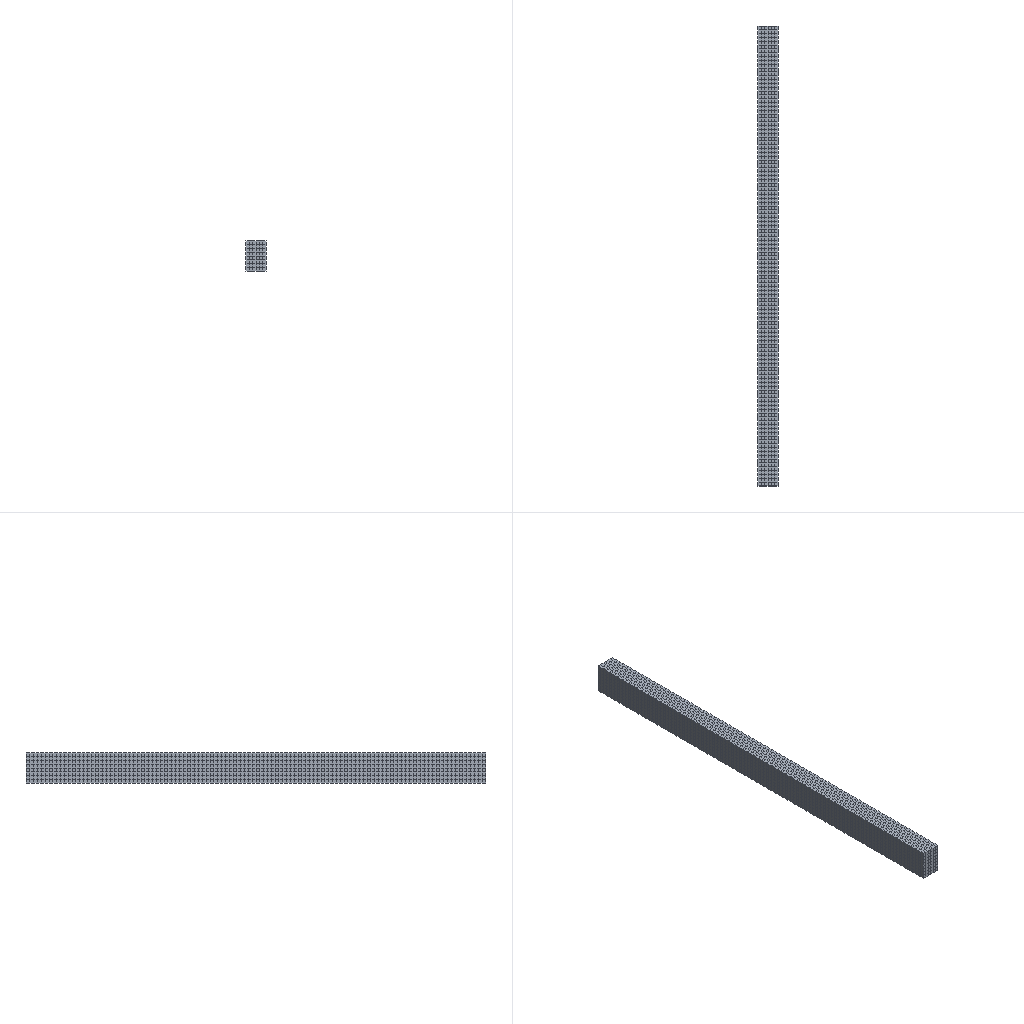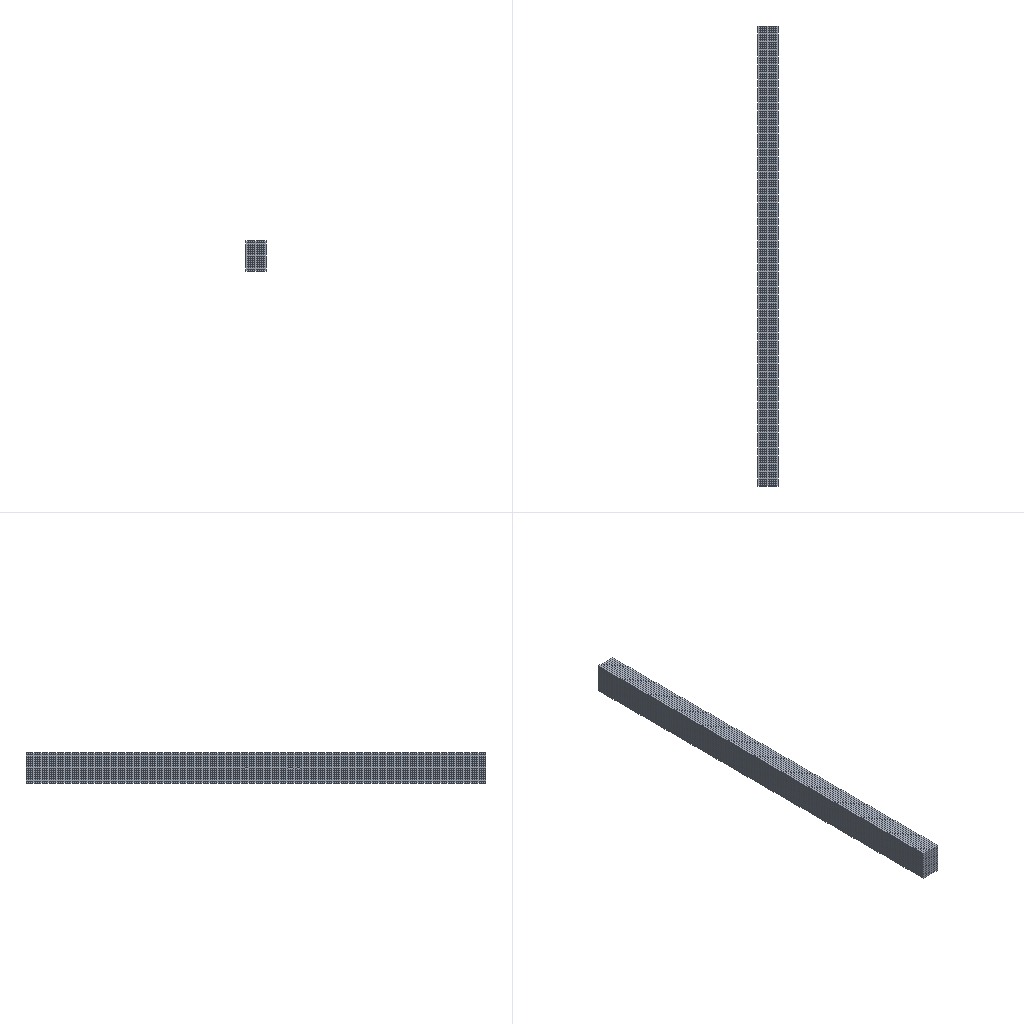Simulation study | ansys workbench
Set-up summary:
category,name,step,type,value,unit,region
solver,ansys_mapdl
solver,version,,,22.1
solver,version,,,22.1
units,MPA,,stated
analysis,deck1,,static,static
load_step,requested,,,1
analysis,nlgeom,,,False
mesh,nodes,,,116275
mesh,elements,,,26568
element_type,ANSYS 186 (type 1),,solid,10080
element_type,ANSYS 186 (type 2),,solid,5040
element_type,ANSYS 186 (type 3),,solid,10080
element_type,ANSYS 174 (type 4),,contact,252
element_type,ANSYS 170 (type 5),,target,252
element_type,ANSYS 174 (type 6),,contact,252
element_type,ANSYS 170 (type 7),,target,252
element_type,ANSYS 154 (type 8),,surface,360
load,load commands in deck,,count,3
bc,support commands in deck,,count,3
named_set,_DISPZEROUX,,component
named_set,_DISPZEROUZ,,component
named_set,_FIXEDSU,,component
analysis,deck2,,static,static
load_step,requested,,,1
analysis,nlgeom,,,False
mesh,nodes,,,28493
mesh,elements,,,6480
element_type,ANSYS 186 (type 1),,solid,5760
element_type,ANSYS 154 (type 2),,surface,720
load,load commands in deck,,count,3
bc,support commands in deck,,count,3
named_set,_DISPZEROUX,,component
named_set,_DISPZEROUZ,,component
named_set,_FIXEDSU,,component
material,1,,in results
material,2,,in results
material,3,,in results
material,1,,in results
check,setup vs results,,match,360 surface effect element(s) are not in the reader's mesh and were not compared
check,setup vs results,,match,720 surface effect element(s) are not in the reader's mesh and were not compared
Results summary:
result,analysis,,,static
result,last_loadstep,,,1
result,primary field,,,displacement
result,reaction total,1,FX,1.2e-05,N
result,reaction total,1,FY,2.2e-05,N
result,reaction total,1,FZ,33000,N
result,mass,,,0.6155,"NMM: mm, ton, N, s, mV, mA, degC"
result,analysis,,,static
result,last_loadstep,,,1
result,primary field,,,displacement
result,reaction total,1,FX,8e-06,N
result,reaction total,1,FY,-3.4e-05,N
result,reaction total,1,FZ,33000,N
result,mass,,,0.6155,"NMM: mm, ton, N, s, mV, mA, degC"